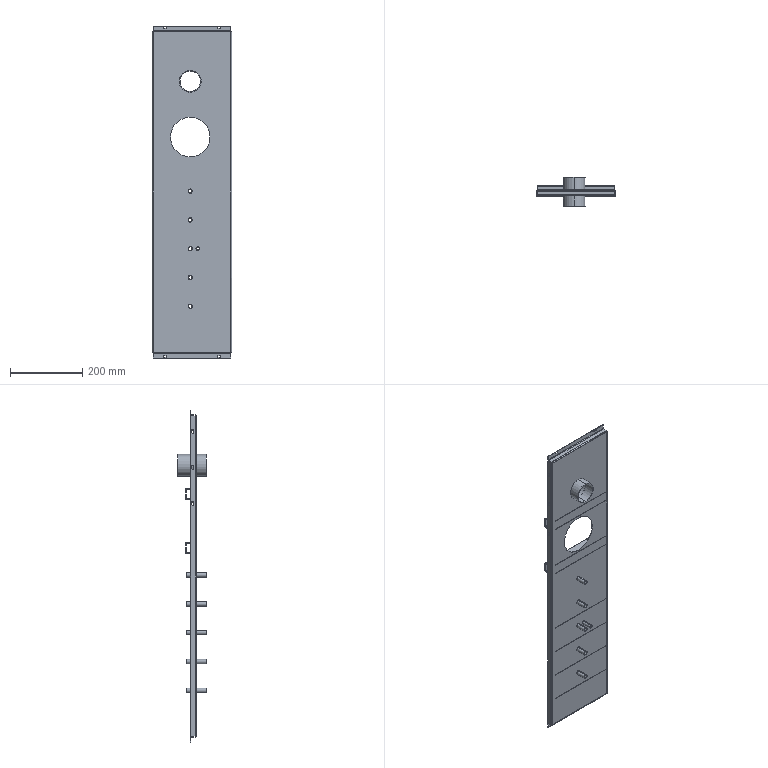Part | STEP file | Sealing plate cover 02001 | 14 solids | 232 faces | box 220 x 80 x 922 mm | volume 432761 mm3 | plane 136 | cylinder 88 | spline 8 | commonest cylinder face diameters 3.5 x24 12 x20 10 x14 3 x10 6 x10 61 x4